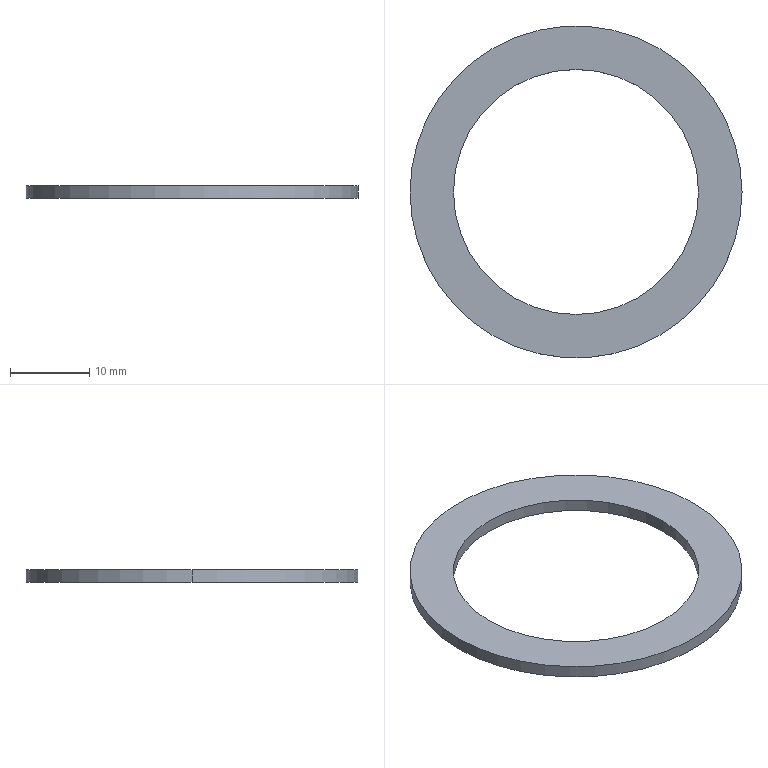Part | SolidWorks | features RefAxis 3, BaseBody 1 | 1 solid | 6 faces | box 42 x 42 x 1.6 mm | volume 1009 mm3 | cylinder 4 | plane 2 | commonest cylinder face diameters 31 x2 42 x2
STEP:
#1=CARTESIAN_POINT('',(15.5,0.,1.6));
#2=VERTEX_POINT('',#1);
#3=CARTESIAN_POINT('',(-15.5,0.,1.6));
#4=VERTEX_POINT('',#3);
#5=CARTESIAN_POINT('',(0.,0.,1.6));
#6=DIRECTION('',(0.,0.,-1.));
#7=DIRECTION('',(-1.,0.,0.));
#8=AXIS2_PLACEMENT_3D('',#5,#6,#7);
#9=CIRCLE('',#8,15.5);
#10=EDGE_CURVE('',#2,#4,#9,.T.);
#11=ORIENTED_EDGE('',*,*,#10,.F.);
#12=CARTESIAN_POINT('',(15.5,0.,0.));
#13=VERTEX_POINT('',#12);
#14=CARTESIAN_POINT('',(15.5,0.,1.6));
#15=DIRECTION('',(0.,0.,-1.));
#16=VECTOR('',#15,1000.);
#17=LINE('',#14,#16);
#18=EDGE_CURVE('',#2,#13,#17,.T.);
#19=ORIENTED_EDGE('',*,*,#18,.T.);
#20=CARTESIAN_POINT('',(-15.5,0.,0.));
#21=VERTEX_POINT('',#20);
#22=CARTESIAN_POINT('',(0.,0.,0.));
#23=DIRECTION('',(0.,0.,1.));
#24=DIRECTION('',(-1.,0.,0.));
#25=AXIS2_PLACEMENT_3D('',#22,#23,#24);
#26=CIRCLE('',#25,15.5);
#27=EDGE_CURVE('',#21,#13,#26,.T.);
#28=ORIENTED_EDGE('',*,*,#27,.F.);
#29=CARTESIAN_POINT('',(-15.5,0.,1.6));
#30=DIRECTION('',(0.,0.,-1.));
#31=VECTOR('',#30,1000.);
#32=LINE('',#29,#31);
#33=EDGE_CURVE('',#4,#21,#32,.T.);
#34=ORIENTED_EDGE('',*,*,#33,.F.);
#35=EDGE_LOOP('',(#11,#19,#28,#34));
#36=FACE_OUTER_BOUND('',#35,.T.);
#37=CARTESIAN_POINT('',(0.,0.,1.6));
#38=DIRECTION('',(0.,0.,-1.));
#39=DIRECTION('',(-1.,0.,0.));
#40=AXIS2_PLACEMENT_3D('',#37,#38,#39);
#41=CYLINDRICAL_SURFACE('',#40,15.5);
#42=ADVANCED_FACE('',(#36),#41,.F.);
#43=CARTESIAN_POINT('',(21.,0.,1.6));
#44=VERTEX_POINT('',#43);
#45=CARTESIAN_POINT('',(-21.,0.,1.6));
#46=VERTEX_POINT('',#45);
#47=CARTESIAN_POINT('',(0.,0.,1.6));
#48=DIRECTION('',(0.,0.,1.));
#49=DIRECTION('',(-1.,0.,0.));
#50=AXIS2_PLACEMENT_3D('',#47,#48,#49);
#51=CIRCLE('',#50,21.);
#52=EDGE_CURVE('',#44,#46,#51,.T.);
#53=ORIENTED_EDGE('',*,*,#52,.F.);
#54=CARTESIAN_POINT('',(21.,0.,0.));
#55=VERTEX_POINT('',#54);
#56=CARTESIAN_POINT('',(21.,0.,1.6));
#57=DIRECTION('',(0.,0.,-1.));
#58=VECTOR('',#57,1000.);
#59=LINE('',#56,#58);
#60=EDGE_CURVE('',#44,#55,#59,.T.);
#61=ORIENTED_EDGE('',*,*,#60,.T.);
#62=CARTESIAN_POINT('',(-21.,0.,0.));
#63=VERTEX_POINT('',#62);
#64=CARTESIAN_POINT('',(0.,0.,0.));
#65=DIRECTION('',(0.,0.,1.));
#66=DIRECTION('',(-1.,0.,0.));
#67=AXIS2_PLACEMENT_3D('',#64,#65,#66);
#68=CIRCLE('',#67,21.);
#69=EDGE_CURVE('',#55,#63,#68,.T.);
#70=ORIENTED_EDGE('',*,*,#69,.T.);
#71=CARTESIAN_POINT('',(-21.,0.,1.6));
#72=DIRECTION('',(0.,0.,-1.));
#73=VECTOR('',#72,1000.);
#74=LINE('',#71,#73);
#75=EDGE_CURVE('',#46,#63,#74,.T.);
#76=ORIENTED_EDGE('',*,*,#75,.F.);
#77=EDGE_LOOP('',(#53,#61,#70,#76));
#78=FACE_OUTER_BOUND('',#77,.T.);
#79=CARTESIAN_POINT('',(0.,0.,1.6));
#80=DIRECTION('',(0.,0.,-1.));
#81=DIRECTION('',(-1.,0.,0.));
#82=AXIS2_PLACEMENT_3D('',#79,#80,#81);
#83=CYLINDRICAL_SURFACE('',#82,21.);
#84=ADVANCED_FACE('',(#78),#83,.T.);
#85=CARTESIAN_POINT('',(0.,0.,1.6));
#86=DIRECTION('',(0.,0.,-1.));
#87=DIRECTION('',(-1.,0.,0.));
#88=AXIS2_PLACEMENT_3D('',#85,#86,#87);
#89=CIRCLE('',#88,15.5);
#90=EDGE_CURVE('',#4,#2,#89,.T.);
#91=ORIENTED_EDGE('',*,*,#90,.T.);
#92=ORIENTED_EDGE('',*,*,#10,.T.);
#93=EDGE_LOOP('',(#91,#92));
#94=FACE_BOUND('',#93,.T.);
#95=CARTESIAN_POINT('',(0.,0.,1.6));
#96=DIRECTION('',(0.,0.,1.));
#97=DIRECTION('',(-1.,0.,0.));
#98=AXIS2_PLACEMENT_3D('',#95,#96,#97);
#99=CIRCLE('',#98,21.);
#100=EDGE_CURVE('',#46,#44,#99,.T.);
#101=ORIENTED_EDGE('',*,*,#100,.T.);
#102=ORIENTED_EDGE('',*,*,#52,.T.);
#103=EDGE_LOOP('',(#101,#102));
#104=FACE_OUTER_BOUND('',#103,.T.);
#105=CARTESIAN_POINT('',(0.,0.,1.6));
#106=DIRECTION('',(0.,0.,1.));
#107=DIRECTION('',(1.,0.,0.));
#108=AXIS2_PLACEMENT_3D('',#105,#106,#107);
#109=PLANE('',#108);
#110=ADVANCED_FACE('',(#94,#104),#109,.T.);
#111=ORIENTED_EDGE('',*,*,#18,.F.);
#112=ORIENTED_EDGE('',*,*,#90,.F.);
#113=ORIENTED_EDGE('',*,*,#33,.T.);
#114=CARTESIAN_POINT('',(0.,0.,0.));
#115=DIRECTION('',(0.,0.,1.));
#116=DIRECTION('',(-1.,0.,0.));
#117=AXIS2_PLACEMENT_3D('',#114,#115,#116);
#118=CIRCLE('',#117,15.5);
#119=EDGE_CURVE('',#13,#21,#118,.T.);
#120=ORIENTED_EDGE('',*,*,#119,.F.);
#121=EDGE_LOOP('',(#111,#112,#113,#120));
#122=FACE_OUTER_BOUND('',#121,.T.);
#123=CARTESIAN_POINT('',(0.,0.,1.6));
#124=DIRECTION('',(0.,0.,-1.));
#125=DIRECTION('',(-1.,0.,0.));
#126=AXIS2_PLACEMENT_3D('',#123,#124,#125);
#127=CYLINDRICAL_SURFACE('',#126,15.5);
#128=ADVANCED_FACE('',(#122),#127,.F.);
#129=ORIENTED_EDGE('',*,*,#60,.F.);
#130=ORIENTED_EDGE('',*,*,#100,.F.);
#131=ORIENTED_EDGE('',*,*,#75,.T.);
#132=CARTESIAN_POINT('',(0.,0.,0.));
#133=DIRECTION('',(0.,0.,1.));
#134=DIRECTION('',(-1.,0.,0.));
#135=AXIS2_PLACEMENT_3D('',#132,#133,#134);
#136=CIRCLE('',#135,21.);
#137=EDGE_CURVE('',#63,#55,#136,.T.);
#138=ORIENTED_EDGE('',*,*,#137,.T.);
#139=EDGE_LOOP('',(#129,#130,#131,#138));
#140=FACE_OUTER_BOUND('',#139,.T.);
#141=CARTESIAN_POINT('',(0.,0.,1.6));
#142=DIRECTION('',(0.,0.,-1.));
#143=DIRECTION('',(-1.,0.,0.));
#144=AXIS2_PLACEMENT_3D('',#141,#142,#143);
#145=CYLINDRICAL_SURFACE('',#144,21.);
#146=ADVANCED_FACE('',(#140),#145,.T.);
#147=ORIENTED_EDGE('',*,*,#27,.T.);
#148=ORIENTED_EDGE('',*,*,#119,.T.);
#149=EDGE_LOOP('',(#147,#148));
#150=FACE_BOUND('',#149,.T.);
#151=ORIENTED_EDGE('',*,*,#137,.F.);
#152=ORIENTED_EDGE('',*,*,#69,.F.);
#153=EDGE_LOOP('',(#151,#152));
#154=FACE_OUTER_BOUND('',#153,.T.);
#155=CARTESIAN_POINT('',(0.,0.,0.));
#156=DIRECTION('',(0.,0.,1.));
#157=DIRECTION('',(1.,0.,0.));
#158=AXIS2_PLACEMENT_3D('',#155,#156,#157);
#159=PLANE('',#158);
#160=ADVANCED_FACE('',(#150,#154),#159,.F.);
#161=CLOSED_SHELL('',(#42,#84,#110,#128,#146,#160));
#162=MANIFOLD_SOLID_BREP('',#161);
#163=CARTESIAN_POINT('',(0.,0.,0.));
#164=DIRECTION('',(0.,0.,1.));
#165=DIRECTION('',(1.,0.,0.));
#166=AXIS2_PLACEMENT_3D('',#163,#164,#165);
#167=(LENGTH_UNIT()NAMED_UNIT(*)SI_UNIT(.MILLI.,.METRE.));
#168=UNCERTAINTY_MEASURE_WITH_UNIT(LENGTH_MEASURE(0.00001),#167,'','');
#169=(NAMED_UNIT(*)PLANE_ANGLE_UNIT()SI_UNIT($,.RADIAN.));
#170=(NAMED_UNIT(*)SI_UNIT($,.STERADIAN.)SOLID_ANGLE_UNIT());
#171=(GEOMETRIC_REPRESENTATION_CONTEXT(3)GLOBAL_UNCERTAINTY_ASSIGNED_CONTEXT((#168))GLOBAL_UNIT_ASSIGNED_CONTEXT((#167,#169,#170))REPRESENTATION_CONTEXT('',''));
#172=ADVANCED_BREP_SHAPE_REPRESENTATION('',(#162,#166),#171);